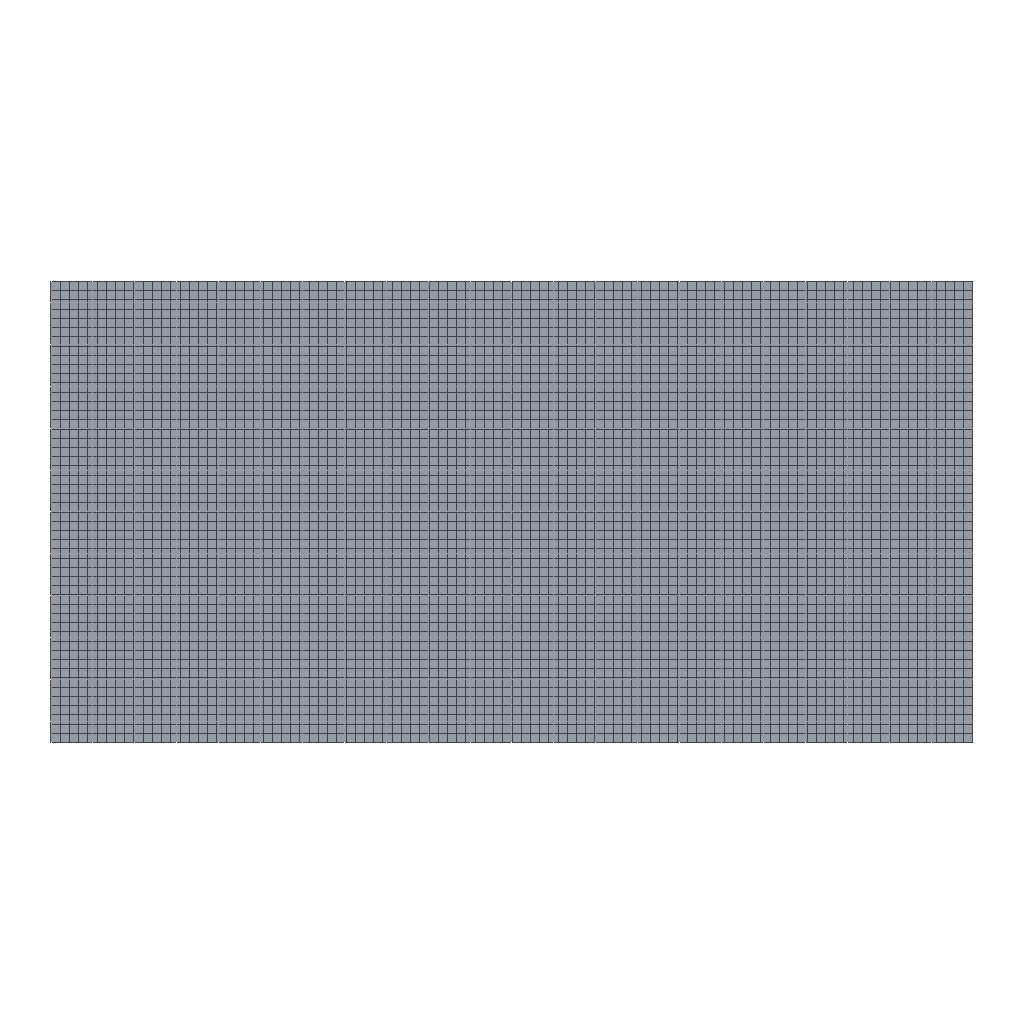Simulation study | abaqus
Set-up summary:
category,name,step,type,value,unit,region
solver,abaqus,,Abaqus/CAE 2024
units,SI m-kg-s (Pa),,inferred,E=1.08e+11 density=4440
analysis,Step-1,,dynamic explicit,nlgeom=True; time_period=0.001075
mesh,nodes,,,10303
mesh,elements,,,10000
element_type,CPE4RT,,,10000
material,TC4,,E,1.08e+11
material,TC4,,nu,0.33
material,TC4,,density,4440
material,TC4,,conductivity,7.5
material,TC4,,cte,9.1e-06
material,TC4,,behaviors,conductivity; damage initiation; damage evolution; expansion
section,TC4,,solid section,,,Set-5
bc,BC-1,Step-1,velocity,"-2 [dofs=rz,x,y n=3]",,Set-6
bc,BC-2,Step-1,encastre,[dofs=ENCASTRE],,Set-7
contact,Int-1,Step-1,contact pair,interaction=IntProp-1; friction=0.4; behavior=hard,,tool-1.RigidSurface_ / s_Set-6_CNS_
constraint,rigid body,,,1
Abaqus input file, long lists of numbers shortened:
*Heading
** Job name: deck Model name: Model-1
** Generated by: Abaqus/CAE 2024
*Preprint, echo=NO, model=NO, history=NO, contact=NO
**
** PARTS
**
*Part, name=tool
*End Part
**
*Part, name=workpiece-mesh-1
*Node
      1, -0.002, -1.92086754e-12
      2, -0.002, -2.00000013e-05
** (5149 more lines like these left out)
*Element, type=CPE4RT
   1,    1,    2,   53,   52
   2,    2,    3,   54,   53
** (4998 more lines like these left out)
*Nset, nset=Set-5, generate
    1,  5151,     1
*Elset, elset=Set-5, generate
    1,  5000,     1
** Section: Section-TC4
*Solid Section, elset=Set-5, controls=EC-1, material=TC4
0.002,
*End Part
**
**
** ASSEMBLY
**
*Assembly, name=Assembly
**
*Instance, name=tool-1, part=tool
9.99999999999998e-05,      -0.0002,           0.
*Node
      1, 0.0006, 0.000975,           0.
*Nset, nset=tool-1-RefPt_, internal
1,
*Surface, type=SEGMENTS, name=RigidSurface_, internal
START,           0.,           0.
 LINE, 0.0006, 6.30625356458706e-05
 LINE, 0.0006,     0.000975
 LINE,           0.,     0.000975
 LINE,           0.,           0.
*End Instance
**
*Instance, name=workpiece-mesh-1-1, part=workpiece-mesh-1
*End Instance
**
*Instance, name=workpiece-mesh-1-2, part=workpiece-mesh-1
*End Instance
**
*Nset, nset=Set-1, instance=tool-1
 1,
*Nset, nset=Set-6, instance=tool-1
 1,
*Nset, nset=Set-7, instance=workpiece-mesh-1-1
   22,   23,   24,   25,   26,   27,   28,   29,   30,   31,   32,   33,   34,   35,   36,   37
   38,   39,   40,   41,   42,   43,   44,   45,   46,   47,   48,   49,   50,   51,   73,   74
** (30 more lines like these left out)
*Nset, nset=Set-7, instance=workpiece-mesh-1-2
   22,   23,   24,   25,   26,   27,   28,   29,   30,   31,   32,   33,   34,   35,   36,   37
   38,   39,   40,   41,   42,   43,   44,   45,   46,   47,   48,   49,   50,   51,   73,   74
** (30 more lines like these left out)
*Nset, nset=s_Set-6, instance=workpiece-mesh-1-1
    1,    2,    3,    4,    5,    6,    7,    8,    9,   10,   11,   12,   13,   14,   52,   53
   54,   55,   56,   57,   58,   59,   60,   61,   62,   63,   64,   65,  103,  104,  105,  106
** (87 more lines like these left out)
*Nset, nset=s_Set-6, instance=workpiece-mesh-1-2
    1,    2,    3,    4,    5,    6,    7,    8,    9,   10,   11,   12,   13,   14,   52,   53
   54,   55,   56,   57,   58,   59,   60,   61,   62,   63,   64,   65,  103,  104,  105,  106
** (87 more lines like these left out)
*Nset, nset=_PickedSet14, internal, instance=tool-1
 1,
*Nset, nset=_PickedSet17, internal, instance=tool-1
 1,
*Surface, type=NODE, name=s_Set-6_CNS_, internal
s_Set-6, 1.
** Constraint: Constraint-1
*Rigid Body, ref node=_PickedSet17, analytical surface=tool-1.RigidSurface_
*End Assembly
**
** ELEMENT CONTROLS
**
*Section Controls, name=EC-1, second order accuracy=YES
1., 1., 1.
*Amplitude, name=Amp-1
             0.,              0.,          0.0001,              1.,          0.0019,              1.,           0.002,              0.
**
** MATERIALS
**
*Material, name=TC4
*Conductivity
  7.5, 20.
  8.7,200.
 11.8,500.
*Damage Initiation, criterion=JOHNSON COOK
 -0.09,  0.25,  -0.5, 0.014,  3.87, 1650.,   25.,    1.
*Damage Evolution, type=DISPLACEMENT
 8e-05,
*Density
4440.,
*Elastic
 1.08e+11, 0.33
*Expansion
 9.1e-06, 20.
 9.2e-06,250.
 9.7e-06,500.
*Inelastic Heat Fraction
         0.9,
*Plastic, hardening=JOHNSON COOK
 8.6e+08, 6.83e+08,     0.47,       1.,    1650.,      25.
*Rate Dependent, type=JOHNSON COOK
 0.035,1.
*Specific Heat
 526.3,
**
** INTERACTION PROPERTIES
**
*Surface Interaction, name=IntProp-1
*Friction
 0.4,
*Surface Behavior, pressure-overclosure=HARD
*Gap Heat Generation
1., 0.5
** ----------------------------------------------------------------
**
** STEP: Step-1
**
*Step, name=Step-1, nlgeom=YES
*Dynamic, Explicit, adiabatic
, 0.001075
*Bulk Viscosity
0.06, 1.2
** Mass Scaling: Semi-Automatic
**               Whole Model
*Fixed Mass Scaling, factor=200.
**
** BOUNDARY CONDITIONS
**
** Name: BC-1 Type: Velocity/Angular velocity
*Boundary, amplitude=Amp-1, type=VELOCITY
Set-6, 1, 1, -2.
Set-6, 2, 2
Set-6, 6, 6
** Name: BC-2 Type: Symmetry/Antisymmetry/Encastre
*Boundary
Set-7, ENCASTRE
**
** INTERACTIONS
**
** Interaction: Int-1
*Contact Pair, interaction=IntProp-1, mechanical constraint=KINEMATIC, cpset=Int-1
tool-1.RigidSurface_, s_Set-6_CNS_
**
** OUTPUT REQUESTS
**
*Restart, write, number interval=1, time marks=NO
**
** FIELD OUTPUT: F-Output-1
**
*Output, field, number interval=100
*Node Output
A, RF, U, V
*Element Output, directions=YES
EVF, LE, PE, PEEQ, PEEQVAVG, PEVAVG, S, STATUS, SVAVG
*Output, history, frequency=0
*End Step
Results summary:
result,odb.job_status,,,JOB_STATUS_COMPLETED_SUCCESSFULLY,"consistent, unstated (Abaqus has no unit system)"
result,steps[0].procedure,Step-1,,"*DYNAMIC, EXPLICIT","consistent, unstated (Abaqus has no unit system)"
result,steps[0].time_period,Step-1,,0.001075,"consistent, unstated (Abaqus has no unit system)"
result,steps[0].n_frames,Step-1,,101,"consistent, unstated (Abaqus has no unit system)"
result,steps[0].last_frame.id,Step-1,,79440,"consistent, unstated (Abaqus has no unit system)"
result,steps[0].last_frame.value,Step-1,,0.001075,"consistent, unstated (Abaqus has no unit system)"
result,steps[0].last_frame.description,Step-1,,Increment     79440: Step Time =   1.0750E-03,"consistent, unstated (Abaqus has no unit system)"
result,steps[0].completed,Step-1,,True,"consistent, unstated (Abaqus has no unit system)"
result,steps[0].max_U_magnitude,Step-1,,0.01868,"consistent, unstated (Abaqus has no unit system)"
result,steps[0].max_S_mises,Step-1,,1.37028e+09,"consistent, unstated (Abaqus has no unit system)"
result,steps[0].RF_sum[1],Step-1,,76.949,"consistent, unstated (Abaqus has no unit system)"
result,steps[0].RF_sum[2],Step-1,,92.462,"consistent, unstated (Abaqus has no unit system)"
result,steps[0].diagnostic.n_increments,Step-1,,101,"consistent, unstated (Abaqus has no unit system)"